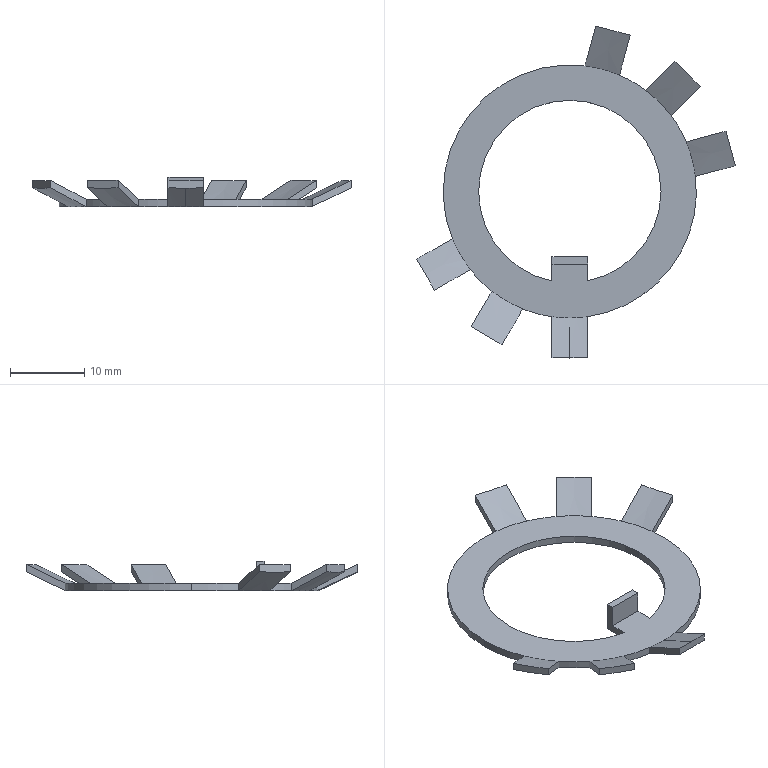Part | SolidWorks | features Boss 1, Cut 1, Revolution 1 | 1 solid | 49 faces | box 42.805 x 44.602 x 4 mm | volume 623.641 mm3 | plane 25 | cone 14 | cylinder 10 | commonest cylinder face diameters 34 x7 24.5 x3
STEP:
#1=CARTESIAN_POINT('',(0.,-17.,0.));
#2=VERTEX_POINT('',#1);
#3=CARTESIAN_POINT('',(-2.4,-16.83,0.));
#4=VERTEX_POINT('',#3);
#5=CARTESIAN_POINT('',(0.,0.,0.));
#6=DIRECTION('',(0.,0.,-1.));
#7=DIRECTION('',(0.,1.,0.));
#8=AXIS2_PLACEMENT_3D('',#5,#6,#7);
#9=CIRCLE('',#8,17.);
#10=EDGE_CURVE('',#2,#4,#9,.T.);
#11=ORIENTED_EDGE('',*,*,#10,.F.);
#12=CARTESIAN_POINT('',(0.,-22.372,2.505));
#13=VERTEX_POINT('',#12);
#14=CARTESIAN_POINT('',(0.,-17.,0.));
#15=DIRECTION('',(0.,-0.9063,0.4226));
#16=VECTOR('',#15,1000.);
#17=LINE('',#14,#16);
#18=EDGE_CURVE('',#2,#13,#17,.T.);
#19=ORIENTED_EDGE('',*,*,#18,.T.);
#20=CARTESIAN_POINT('',(-2.4,-22.372,2.565));
#21=VERTEX_POINT('',#20);
#22=CARTESIAN_POINT('',(0.,-22.372,2.505));
#23=CARTESIAN_POINT('',(-0.7988,-22.372,2.505));
#24=CARTESIAN_POINT('',(-1.6,-22.372,2.525));
#25=CARTESIAN_POINT('',(-2.4,-22.372,2.565));
#26=B_SPLINE_CURVE_WITH_KNOTS('',3,(#22,#23,#24,#25),.UNSPECIFIED.,.F.,.F.,(4,4),(0.00905,0.01144),.UNSPECIFIED.);
#27=EDGE_CURVE('',#13,#21,#26,.T.);
#28=ORIENTED_EDGE('',*,*,#27,.T.);
#29=CARTESIAN_POINT('',(-2.4,-22.372,2.565));
#30=CARTESIAN_POINT('',(-2.4,-20.525,1.708));
#31=CARTESIAN_POINT('',(-2.4,-18.678,0.8532));
#32=CARTESIAN_POINT('',(-2.4,-16.83,0.));
#33=B_SPLINE_CURVE_WITH_KNOTS('',3,(#29,#30,#31,#32),.UNSPECIFIED.,.F.,.F.,(4,4),(0.01129,0.01739),.UNSPECIFIED.);
#34=EDGE_CURVE('',#21,#4,#33,.T.);
#35=ORIENTED_EDGE('',*,*,#34,.T.);
#36=EDGE_LOOP('',(#11,#19,#28,#35));
#37=FACE_OUTER_BOUND('',#36,.T.);
#38=CARTESIAN_POINT('',(0.,0.,0.));
#39=DIRECTION('',(0.,0.,1.));
#40=DIRECTION('',(0.,-1.,0.));
#41=AXIS2_PLACEMENT_3D('',#38,#39,#40);
#42=CONICAL_SURFACE('',#41,17.,1.134);
#43=ADVANCED_FACE('',(#37),#42,.T.);
#44=CARTESIAN_POINT('',(-15.775,-6.336,1.));
#45=VERTEX_POINT('',#44);
#46=CARTESIAN_POINT('',(-17.,0.,1.));
#47=VERTEX_POINT('',#46);
#48=CARTESIAN_POINT('',(0.,0.,1.));
#49=DIRECTION('',(0.,0.,-1.));
#50=DIRECTION('',(0.,1.,0.));
#51=AXIS2_PLACEMENT_3D('',#48,#49,#50);
#52=CIRCLE('',#51,17.);
#53=EDGE_CURVE('',#45,#47,#52,.T.);
#54=ORIENTED_EDGE('',*,*,#53,.T.);
#55=CARTESIAN_POINT('',(-17.,0.,0.));
#56=VERTEX_POINT('',#55);
#57=CARTESIAN_POINT('',(-17.,0.,3.566));
#58=DIRECTION('',(0.,0.,-1.));
#59=VECTOR('',#58,1000.);
#60=LINE('',#57,#59);
#61=EDGE_CURVE('',#47,#56,#60,.T.);
#62=ORIENTED_EDGE('',*,*,#61,.T.);
#63=CARTESIAN_POINT('',(-15.775,-6.336,0.));
#64=VERTEX_POINT('',#63);
#65=CARTESIAN_POINT('',(0.,0.,0.));
#66=DIRECTION('',(0.,0.,1.));
#67=DIRECTION('',(1.,0.,0.));
#68=AXIS2_PLACEMENT_3D('',#65,#66,#67);
#69=CIRCLE('',#68,17.);
#70=EDGE_CURVE('',#56,#64,#69,.T.);
#71=ORIENTED_EDGE('',*,*,#70,.T.);
#72=CARTESIAN_POINT('',(-15.775,-6.336,3.566));
#73=DIRECTION('',(0.,0.,-1.));
#74=VECTOR('',#73,1000.);
#75=LINE('',#72,#74);
#76=EDGE_CURVE('',#45,#64,#75,.T.);
#77=ORIENTED_EDGE('',*,*,#76,.F.);
#78=EDGE_LOOP('',(#54,#62,#71,#77));
#79=FACE_OUTER_BOUND('',#78,.T.);
#80=CARTESIAN_POINT('',(0.,0.,3.566));
#81=DIRECTION('',(0.,0.,-1.));
#82=DIRECTION('',(-1.,0.,0.));
#83=AXIS2_PLACEMENT_3D('',#80,#81,#82);
#84=CYLINDRICAL_SURFACE('',#83,17.);
#85=ADVANCED_FACE('',(#79),#84,.T.);
#86=CARTESIAN_POINT('',(2.4,-12.013,1.));
#87=VERTEX_POINT('',#86);
#88=CARTESIAN_POINT('',(12.25,0.,1.));
#89=VERTEX_POINT('',#88);
#90=CARTESIAN_POINT('',(0.,0.,1.));
#91=DIRECTION('',(0.,0.,1.));
#92=DIRECTION('',(0.,-1.,0.));
#93=AXIS2_PLACEMENT_3D('',#90,#91,#92);
#94=CIRCLE('',#93,12.25);
#95=EDGE_CURVE('',#87,#89,#94,.T.);
#96=ORIENTED_EDGE('',*,*,#95,.T.);
#97=CARTESIAN_POINT('',(12.25,0.,0.));
#98=VERTEX_POINT('',#97);
#99=CARTESIAN_POINT('',(12.25,0.,3.566));
#100=DIRECTION('',(0.,0.,-1.));
#101=VECTOR('',#100,1000.);
#102=LINE('',#99,#101);
#103=EDGE_CURVE('',#89,#98,#102,.T.);
#104=ORIENTED_EDGE('',*,*,#103,.T.);
#105=CARTESIAN_POINT('',(2.4,-12.013,0.));
#106=VERTEX_POINT('',#105);
#107=CARTESIAN_POINT('',(0.,0.,0.));
#108=DIRECTION('',(0.,0.,1.));
#109=DIRECTION('',(1.,0.,0.));
#110=AXIS2_PLACEMENT_3D('',#107,#108,#109);
#111=CIRCLE('',#110,12.25);
#112=EDGE_CURVE('',#106,#98,#111,.T.);
#113=ORIENTED_EDGE('',*,*,#112,.F.);
#114=CARTESIAN_POINT('',(2.4,-12.013,3.566));
#115=DIRECTION('',(0.,0.,-1.));
#116=VECTOR('',#115,1000.);
#117=LINE('',#114,#116);
#118=EDGE_CURVE('',#87,#106,#117,.T.);
#119=ORIENTED_EDGE('',*,*,#118,.F.);
#120=EDGE_LOOP('',(#96,#104,#113,#119));
#121=FACE_OUTER_BOUND('',#120,.T.);
#122=CARTESIAN_POINT('',(0.,0.,3.566));
#123=DIRECTION('',(0.,0.,-1.));
#124=DIRECTION('',(-1.,0.,0.));
#125=AXIS2_PLACEMENT_3D('',#122,#123,#124);
#126=CYLINDRICAL_SURFACE('',#125,12.25);
#127=ADVANCED_FACE('',(#121),#126,.F.);
#128=ORIENTED_EDGE('',*,*,#103,.F.);
#129=CARTESIAN_POINT('',(-12.25,0.,1.));
#130=VERTEX_POINT('',#129);
#131=CARTESIAN_POINT('',(0.,0.,1.));
#132=DIRECTION('',(0.,0.,1.));
#133=DIRECTION('',(0.,-1.,0.));
#134=AXIS2_PLACEMENT_3D('',#131,#132,#133);
#135=CIRCLE('',#134,12.25);
#136=EDGE_CURVE('',#89,#130,#135,.T.);
#137=ORIENTED_EDGE('',*,*,#136,.T.);
#138=CARTESIAN_POINT('',(-12.25,0.,0.));
#139=VERTEX_POINT('',#138);
#140=CARTESIAN_POINT('',(-12.25,0.,3.566));
#141=DIRECTION('',(0.,0.,-1.));
#142=VECTOR('',#141,1000.);
#143=LINE('',#140,#142);
#144=EDGE_CURVE('',#130,#139,#143,.T.);
#145=ORIENTED_EDGE('',*,*,#144,.T.);
#146=CARTESIAN_POINT('',(0.,0.,0.));
#147=DIRECTION('',(0.,0.,1.));
#148=DIRECTION('',(1.,0.,0.));
#149=AXIS2_PLACEMENT_3D('',#146,#147,#148);
#150=CIRCLE('',#149,12.25);
#151=EDGE_CURVE('',#98,#139,#150,.T.);
#152=ORIENTED_EDGE('',*,*,#151,.F.);
#153=EDGE_LOOP('',(#128,#137,#145,#152));
#154=FACE_OUTER_BOUND('',#153,.T.);
#155=CARTESIAN_POINT('',(0.,0.,3.566));
#156=DIRECTION('',(0.,0.,-1.));
#157=DIRECTION('',(-1.,0.,0.));
#158=AXIS2_PLACEMENT_3D('',#155,#156,#157);
#159=CYLINDRICAL_SURFACE('',#158,12.25);
#160=ADVANCED_FACE('',(#154),#159,.F.);
#161=CARTESIAN_POINT('',(2.4,-16.83,1.));
#162=VERTEX_POINT('',#161);
#163=CARTESIAN_POINT('',(0.,-17.,1.));
#164=VERTEX_POINT('',#163);
#165=CARTESIAN_POINT('',(0.,0.,1.));
#166=DIRECTION('',(0.,0.,-1.));
#167=DIRECTION('',(0.,1.,0.));
#168=AXIS2_PLACEMENT_3D('',#165,#166,#167);
#169=CIRCLE('',#168,17.);
#170=EDGE_CURVE('',#162,#164,#169,.T.);
#171=ORIENTED_EDGE('',*,*,#170,.T.);
#172=CARTESIAN_POINT('',(0.,-22.372,3.505));
#173=VERTEX_POINT('',#172);
#174=CARTESIAN_POINT('',(0.,-22.5,3.565));
#175=DIRECTION('',(0.,-0.9063,0.4226));
#176=VECTOR('',#175,1000.);
#177=LINE('',#174,#176);
#178=EDGE_CURVE('',#164,#173,#177,.T.);
#179=ORIENTED_EDGE('',*,*,#178,.T.);
#180=CARTESIAN_POINT('',(2.4,-22.372,3.565));
#181=VERTEX_POINT('',#180);
#182=CARTESIAN_POINT('',(0.,-22.372,3.505));
#183=CARTESIAN_POINT('',(0.8014,-22.372,3.505));
#184=CARTESIAN_POINT('',(1.601,-22.372,3.525));
#185=CARTESIAN_POINT('',(2.4,-22.372,3.565));
#186=B_SPLINE_CURVE_WITH_KNOTS('',3,(#182,#183,#184,#185),.UNSPECIFIED.,.F.,.F.,(4,4),(0.01258,0.01498),.UNSPECIFIED.);
#187=EDGE_CURVE('',#173,#181,#186,.T.);
#188=ORIENTED_EDGE('',*,*,#187,.T.);
#189=CARTESIAN_POINT('',(2.4,-22.372,3.565));
#190=CARTESIAN_POINT('',(2.4,-20.525,2.708));
#191=CARTESIAN_POINT('',(2.4,-18.678,1.853));
#192=CARTESIAN_POINT('',(2.4,-16.83,1.));
#193=B_SPLINE_CURVE_WITH_KNOTS('',3,(#189,#190,#191,#192),.UNSPECIFIED.,.F.,.F.,(4,4),(0.01129,0.01739),.UNSPECIFIED.);
#194=EDGE_CURVE('',#181,#162,#193,.T.);
#195=ORIENTED_EDGE('',*,*,#194,.T.);
#196=EDGE_LOOP('',(#171,#179,#188,#195));
#197=FACE_OUTER_BOUND('',#196,.T.);
#198=CARTESIAN_POINT('',(0.,0.,3.565));
#199=DIRECTION('',(0.,0.,1.));
#200=DIRECTION('',(0.,-1.,0.));
#201=AXIS2_PLACEMENT_3D('',#198,#199,#200);
#202=CONICAL_SURFACE('',#201,22.5,1.134);
#203=ADVANCED_FACE('',(#197),#202,.F.);
#204=CARTESIAN_POINT('',(2.038,16.877,1.));
#205=VERTEX_POINT('',#204);
#206=CARTESIAN_POINT('',(6.674,15.635,1.));
#207=VERTEX_POINT('',#206);
#208=CARTESIAN_POINT('',(0.,0.,1.));
#209=DIRECTION('',(0.,0.,-1.));
#210=DIRECTION('',(0.,1.,0.));
#211=AXIS2_PLACEMENT_3D('',#208,#209,#210);
#212=CIRCLE('',#211,17.);
#213=EDGE_CURVE('',#205,#207,#212,.T.);
#214=ORIENTED_EDGE('',*,*,#213,.F.);
#215=CARTESIAN_POINT('',(0.,0.,1.));
#216=DIRECTION('',(0.,0.,-1.));
#217=DIRECTION('',(0.,1.,0.));
#218=AXIS2_PLACEMENT_3D('',#215,#216,#217);
#219=CIRCLE('',#218,17.);
#220=EDGE_CURVE('',#47,#205,#219,.T.);
#221=ORIENTED_EDGE('',*,*,#220,.F.);
#222=ORIENTED_EDGE('',*,*,#53,.F.);
#223=CARTESIAN_POINT('',(-13.375,-10.493,1.));
#224=VERTEX_POINT('',#223);
#225=CARTESIAN_POINT('',(0.,0.,1.));
#226=DIRECTION('',(0.,0.,-1.));
#227=DIRECTION('',(0.,1.,0.));
#228=AXIS2_PLACEMENT_3D('',#225,#226,#227);
#229=CIRCLE('',#228,17.);
#230=EDGE_CURVE('',#224,#45,#229,.T.);
#231=ORIENTED_EDGE('',*,*,#230,.F.);
#232=CARTESIAN_POINT('',(-10.493,-13.375,1.));
#233=VERTEX_POINT('',#232);
#234=CARTESIAN_POINT('',(0.,0.,1.));
#235=DIRECTION('',(0.,0.,-1.));
#236=DIRECTION('',(0.,1.,0.));
#237=AXIS2_PLACEMENT_3D('',#234,#235,#236);
#238=CIRCLE('',#237,17.);
#239=EDGE_CURVE('',#233,#224,#238,.T.);
#240=ORIENTED_EDGE('',*,*,#239,.F.);
#241=CARTESIAN_POINT('',(-6.336,-15.775,1.));
#242=VERTEX_POINT('',#241);
#243=CARTESIAN_POINT('',(0.,0.,1.));
#244=DIRECTION('',(0.,0.,-1.));
#245=DIRECTION('',(0.,1.,0.));
#246=AXIS2_PLACEMENT_3D('',#243,#244,#245);
#247=CIRCLE('',#246,17.);
#248=EDGE_CURVE('',#242,#233,#247,.T.);
#249=ORIENTED_EDGE('',*,*,#248,.F.);
#250=CARTESIAN_POINT('',(-2.4,-16.83,1.));
#251=VERTEX_POINT('',#250);
#252=CARTESIAN_POINT('',(0.,0.,1.));
#253=DIRECTION('',(0.,0.,-1.));
#254=DIRECTION('',(0.,1.,0.));
#255=AXIS2_PLACEMENT_3D('',#252,#253,#254);
#256=CIRCLE('',#255,17.);
#257=EDGE_CURVE('',#251,#242,#256,.T.);
#258=ORIENTED_EDGE('',*,*,#257,.F.);
#259=CARTESIAN_POINT('',(0.,0.,1.));
#260=DIRECTION('',(0.,0.,-1.));
#261=DIRECTION('',(0.,1.,0.));
#262=AXIS2_PLACEMENT_3D('',#259,#260,#261);
#263=CIRCLE('',#262,17.);
#264=EDGE_CURVE('',#164,#251,#263,.T.);
#265=ORIENTED_EDGE('',*,*,#264,.F.);
#266=ORIENTED_EDGE('',*,*,#170,.F.);
#267=CARTESIAN_POINT('',(16.877,2.038,1.));
#268=VERTEX_POINT('',#267);
#269=CARTESIAN_POINT('',(0.,0.,1.));
#270=DIRECTION('',(0.,0.,-1.));
#271=DIRECTION('',(0.,1.,0.));
#272=AXIS2_PLACEMENT_3D('',#269,#270,#271);
#273=CIRCLE('',#272,17.);
#274=EDGE_CURVE('',#268,#162,#273,.T.);
#275=ORIENTED_EDGE('',*,*,#274,.F.);
#276=CARTESIAN_POINT('',(15.635,6.674,1.));
#277=VERTEX_POINT('',#276);
#278=CARTESIAN_POINT('',(0.,0.,1.));
#279=DIRECTION('',(0.,0.,-1.));
#280=DIRECTION('',(0.,1.,0.));
#281=AXIS2_PLACEMENT_3D('',#278,#279,#280);
#282=CIRCLE('',#281,17.);
#283=EDGE_CURVE('',#277,#268,#282,.T.);
#284=ORIENTED_EDGE('',*,*,#283,.F.);
#285=CARTESIAN_POINT('',(13.597,10.203,1.));
#286=VERTEX_POINT('',#285);
#287=CARTESIAN_POINT('',(0.,0.,1.));
#288=DIRECTION('',(0.,0.,-1.));
#289=DIRECTION('',(0.,1.,0.));
#290=AXIS2_PLACEMENT_3D('',#287,#288,#289);
#291=CIRCLE('',#290,17.);
#292=EDGE_CURVE('',#286,#277,#291,.T.);
#293=ORIENTED_EDGE('',*,*,#292,.F.);
#294=CARTESIAN_POINT('',(10.203,13.597,1.));
#295=VERTEX_POINT('',#294);
#296=CARTESIAN_POINT('',(0.,0.,1.));
#297=DIRECTION('',(0.,0.,-1.));
#298=DIRECTION('',(0.,1.,0.));
#299=AXIS2_PLACEMENT_3D('',#296,#297,#298);
#300=CIRCLE('',#299,17.);
#301=EDGE_CURVE('',#295,#286,#300,.T.);
#302=ORIENTED_EDGE('',*,*,#301,.F.);
#303=CARTESIAN_POINT('',(0.,0.,1.));
#304=DIRECTION('',(0.,0.,-1.));
#305=DIRECTION('',(0.,1.,0.));
#306=AXIS2_PLACEMENT_3D('',#303,#304,#305);
#307=CIRCLE('',#306,17.);
#308=EDGE_CURVE('',#207,#295,#307,.T.);
#309=ORIENTED_EDGE('',*,*,#308,.F.);
#310=EDGE_LOOP('',(#214,#221,#222,#231,#240,#249,#258,#265,#266,#275,#284,#293,#302,#309));
#311=FACE_OUTER_BOUND('',#310,.T.);
#312=CARTESIAN_POINT('',(2.4,-9.75,1.));
#313=VERTEX_POINT('',#312);
#314=CARTESIAN_POINT('',(2.4,-12.013,1.));
#315=DIRECTION('',(0.,-1.,0.));
#316=VECTOR('',#315,1000.);
#317=LINE('',#314,#316);
#318=EDGE_CURVE('',#313,#87,#317,.T.);
#319=ORIENTED_EDGE('',*,*,#318,.F.);
#320=CARTESIAN_POINT('',(-2.4,-9.75,1.));
#321=VERTEX_POINT('',#320);
#322=CARTESIAN_POINT('',(0.,-9.75,1.));
#323=DIRECTION('',(-1.,0.,0.));
#324=VECTOR('',#323,1000.);
#325=LINE('',#322,#324);
#326=EDGE_CURVE('',#313,#321,#325,.T.);
#327=ORIENTED_EDGE('',*,*,#326,.T.);
#328=CARTESIAN_POINT('',(-2.4,-12.013,1.));
#329=VERTEX_POINT('',#328);
#330=CARTESIAN_POINT('',(-2.4,-12.013,1.));
#331=DIRECTION('',(0.,1.,0.));
#332=VECTOR('',#331,1000.);
#333=LINE('',#330,#332);
#334=EDGE_CURVE('',#329,#321,#333,.T.);
#335=ORIENTED_EDGE('',*,*,#334,.F.);
#336=CARTESIAN_POINT('',(0.,0.,1.));
#337=DIRECTION('',(0.,0.,1.));
#338=DIRECTION('',(0.,-1.,0.));
#339=AXIS2_PLACEMENT_3D('',#336,#337,#338);
#340=CIRCLE('',#339,12.25);
#341=EDGE_CURVE('',#130,#329,#340,.T.);
#342=ORIENTED_EDGE('',*,*,#341,.F.);
#343=ORIENTED_EDGE('',*,*,#136,.F.);
#344=ORIENTED_EDGE('',*,*,#95,.F.);
#345=EDGE_LOOP('',(#319,#327,#335,#342,#343,#344));
#346=FACE_BOUND('',#345,.T.);
#347=CARTESIAN_POINT('',(0.,17.,1.));
#348=DIRECTION('',(0.,0.,1.));
#349=DIRECTION('',(0.,-1.,0.));
#350=AXIS2_PLACEMENT_3D('',#347,#348,#349);
#351=PLANE('',#350);
#352=ADVANCED_FACE('',(#311,#346),#351,.T.);
#353=ORIENTED_EDGE('',*,*,#178,.F.);
#354=ORIENTED_EDGE('',*,*,#264,.T.);
#355=CARTESIAN_POINT('',(-2.4,-22.372,3.565));
#356=VERTEX_POINT('',#355);
#357=CARTESIAN_POINT('',(-2.4,-16.83,1.));
#358=CARTESIAN_POINT('',(-2.4,-18.678,1.853));
#359=CARTESIAN_POINT('',(-2.4,-20.525,2.708));
#360=CARTESIAN_POINT('',(-2.4,-22.372,3.565));
#361=B_SPLINE_CURVE_WITH_KNOTS('',3,(#357,#358,#359,#360),.UNSPECIFIED.,.F.,.F.,(4,4),(0.006977,0.01308),.UNSPECIFIED.);
#362=EDGE_CURVE('',#251,#356,#361,.T.);
#363=ORIENTED_EDGE('',*,*,#362,.T.);
#364=CARTESIAN_POINT('',(-2.4,-22.372,3.565));
#365=CARTESIAN_POINT('',(-1.6,-22.372,3.525));
#366=CARTESIAN_POINT('',(-0.7988,-22.372,3.505));
#367=CARTESIAN_POINT('',(0.,-22.372,3.505));
#368=B_SPLINE_CURVE_WITH_KNOTS('',3,(#364,#365,#366,#367),.UNSPECIFIED.,.F.,.F.,(4,4),(0.01019,0.01258),.UNSPECIFIED.);
#369=EDGE_CURVE('',#356,#173,#368,.T.);
#370=ORIENTED_EDGE('',*,*,#369,.T.);
#371=EDGE_LOOP('',(#353,#354,#363,#370));
#372=FACE_OUTER_BOUND('',#371,.T.);
#373=CARTESIAN_POINT('',(0.,0.,3.565));
#374=DIRECTION('',(0.,0.,1.));
#375=DIRECTION('',(0.,-1.,0.));
#376=AXIS2_PLACEMENT_3D('',#373,#374,#375);
#377=CONICAL_SURFACE('',#376,22.5,1.134);
#378=ADVANCED_FACE('',(#372),#377,.F.);
#379=CARTESIAN_POINT('',(-13.264,-18.174,3.565));
#380=VERTEX_POINT('',#379);
#381=CARTESIAN_POINT('',(-10.493,-13.375,1.));
#382=CARTESIAN_POINT('',(-11.417,-14.975,1.853));
#383=CARTESIAN_POINT('',(-12.341,-16.575,2.708));
#384=CARTESIAN_POINT('',(-13.264,-18.174,3.565));
#385=B_SPLINE_CURVE_WITH_KNOTS('',3,(#381,#382,#383,#384),.UNSPECIFIED.,.F.,.F.,(4,4),(0.000000254,0.006107),.UNSPECIFIED.);
#386=EDGE_CURVE('',#233,#380,#385,.T.);
#387=ORIENTED_EDGE('',*,*,#386,.T.);
#388=CARTESIAN_POINT('',(-9.107,-20.574,3.565));
#389=VERTEX_POINT('',#388);
#390=CARTESIAN_POINT('',(-13.264,-18.174,3.565));
#391=CARTESIAN_POINT('',(-11.879,-18.974,3.485));
#392=CARTESIAN_POINT('',(-10.493,-19.774,3.485));
#393=CARTESIAN_POINT('',(-9.107,-20.574,3.565));
#394=B_SPLINE_CURVE_WITH_KNOTS('',3,(#390,#391,#392,#393),.UNSPECIFIED.,.F.,.F.,(4,4),(0.000000231,0.0048),.UNSPECIFIED.);
#395=EDGE_CURVE('',#380,#389,#394,.T.);
#396=ORIENTED_EDGE('',*,*,#395,.T.);
#397=CARTESIAN_POINT('',(-9.107,-20.574,3.565));
#398=CARTESIAN_POINT('',(-8.184,-18.975,2.708));
#399=CARTESIAN_POINT('',(-7.26,-17.375,1.853));
#400=CARTESIAN_POINT('',(-6.336,-15.775,1.));
#401=B_SPLINE_CURVE_WITH_KNOTS('',3,(#397,#398,#399,#400),.UNSPECIFIED.,.F.,.F.,(4,4),(0.000000255,0.006107),.UNSPECIFIED.);
#402=EDGE_CURVE('',#389,#242,#401,.T.);
#403=ORIENTED_EDGE('',*,*,#402,.T.);
#404=ORIENTED_EDGE('',*,*,#248,.T.);
#405=EDGE_LOOP('',(#387,#396,#403,#404));
#406=FACE_OUTER_BOUND('',#405,.T.);
#407=CARTESIAN_POINT('',(0.,0.,3.565));
#408=DIRECTION('',(0.,0.,1.));
#409=DIRECTION('',(0.,-1.,0.));
#410=AXIS2_PLACEMENT_3D('',#407,#408,#409);
#411=CONICAL_SURFACE('',#410,22.5,1.134);
#412=ADVANCED_FACE('',(#406),#411,.F.);
#413=CARTESIAN_POINT('',(-20.574,-9.107,3.565));
#414=VERTEX_POINT('',#413);
#415=CARTESIAN_POINT('',(-15.775,-6.336,1.));
#416=CARTESIAN_POINT('',(-17.375,-7.26,1.853));
#417=CARTESIAN_POINT('',(-18.975,-8.184,2.708));
#418=CARTESIAN_POINT('',(-20.574,-9.107,3.565));
#419=B_SPLINE_CURVE_WITH_KNOTS('',3,(#415,#416,#417,#418),.UNSPECIFIED.,.F.,.F.,(4,4),(0.000000254,0.006107),.UNSPECIFIED.);
#420=EDGE_CURVE('',#45,#414,#419,.T.);
#421=ORIENTED_EDGE('',*,*,#420,.T.);
#422=CARTESIAN_POINT('',(-18.174,-13.264,3.565));
#423=VERTEX_POINT('',#422);
#424=CARTESIAN_POINT('',(-20.574,-9.107,3.565));
#425=CARTESIAN_POINT('',(-19.774,-10.493,3.485));
#426=CARTESIAN_POINT('',(-18.974,-11.879,3.485));
#427=CARTESIAN_POINT('',(-18.174,-13.264,3.565));
#428=B_SPLINE_CURVE_WITH_KNOTS('',3,(#424,#425,#426,#427),.UNSPECIFIED.,.F.,.F.,(4,4),(0.000000231,0.0048),.UNSPECIFIED.);
#429=EDGE_CURVE('',#414,#423,#428,.T.);
#430=ORIENTED_EDGE('',*,*,#429,.T.);
#431=CARTESIAN_POINT('',(-18.174,-13.264,3.565));
#432=CARTESIAN_POINT('',(-16.575,-12.341,2.708));
#433=CARTESIAN_POINT('',(-14.975,-11.417,1.853));
#434=CARTESIAN_POINT('',(-13.375,-10.493,1.));
#435=B_SPLINE_CURVE_WITH_KNOTS('',3,(#431,#432,#433,#434),.UNSPECIFIED.,.F.,.F.,(4,4),(0.000000255,0.006107),.UNSPECIFIED.);
#436=EDGE_CURVE('',#423,#224,#435,.T.);
#437=ORIENTED_EDGE('',*,*,#436,.T.);
#438=ORIENTED_EDGE('',*,*,#230,.T.);
#439=EDGE_LOOP('',(#421,#430,#437,#438));
#440=FACE_OUTER_BOUND('',#439,.T.);
#441=CARTESIAN_POINT('',(0.,0.,3.565));
#442=DIRECTION('',(0.,0.,1.));
#443=DIRECTION('',(0.,-1.,0.));
#444=AXIS2_PLACEMENT_3D('',#441,#442,#443);
#445=CONICAL_SURFACE('',#444,22.5,1.134);
#446=ADVANCED_FACE('',(#440),#445,.F.);
#447=CARTESIAN_POINT('',(8.108,20.988,3.565));
#448=VERTEX_POINT('',#447);
#449=CARTESIAN_POINT('',(6.674,15.635,1.));
#450=CARTESIAN_POINT('',(7.152,17.42,1.853));
#451=CARTESIAN_POINT('',(7.63,19.204,2.708));
#452=CARTESIAN_POINT('',(8.108,20.988,3.565));
#453=B_SPLINE_CURVE_WITH_KNOTS('',3,(#449,#450,#451,#452),.UNSPECIFIED.,.F.,.F.,(4,4),(0.000000228,0.006107),.UNSPECIFIED.);
#454=EDGE_CURVE('',#207,#448,#453,.T.);
#455=ORIENTED_EDGE('',*,*,#454,.T.);
#456=CARTESIAN_POINT('',(3.472,22.231,3.565));
#457=VERTEX_POINT('',#456);
#458=CARTESIAN_POINT('',(8.108,20.988,3.565));
#459=CARTESIAN_POINT('',(6.563,21.402,3.485));
#460=CARTESIAN_POINT('',(5.017,21.816,3.485));
#461=CARTESIAN_POINT('',(3.472,22.231,3.565));
#462=B_SPLINE_CURVE_WITH_KNOTS('',3,(#458,#459,#460,#461),.UNSPECIFIED.,.F.,.F.,(4,4),(0.000000207,0.0048),.UNSPECIFIED.);
#463=EDGE_CURVE('',#448,#457,#462,.T.);
#464=ORIENTED_EDGE('',*,*,#463,.T.);
#465=CARTESIAN_POINT('',(3.472,22.231,3.565));
#466=CARTESIAN_POINT('',(2.994,20.447,2.708));
#467=CARTESIAN_POINT('',(2.516,18.663,1.853));
#468=CARTESIAN_POINT('',(2.038,16.877,1.));
#469=B_SPLINE_CURVE_WITH_KNOTS('',3,(#465,#466,#467,#468),.UNSPECIFIED.,.F.,.F.,(4,4),(0.000000228,0.006107),.UNSPECIFIED.);
#470=EDGE_CURVE('',#457,#205,#469,.T.);
#471=ORIENTED_EDGE('',*,*,#470,.T.);
#472=ORIENTED_EDGE('',*,*,#213,.T.);
#473=EDGE_LOOP('',(#455,#464,#471,#472));
#474=FACE_OUTER_BOUND('',#473,.T.);
#475=CARTESIAN_POINT('',(0.,0.,3.565));
#476=DIRECTION('',(0.,0.,1.));
#477=DIRECTION('',(0.,-1.,0.));
#478=AXIS2_PLACEMENT_3D('',#475,#476,#477);
#479=CONICAL_SURFACE('',#478,22.5,1.134);
#480=ADVANCED_FACE('',(#474),#479,.F.);
#481=CARTESIAN_POINT('',(17.516,14.122,3.565));
#482=VERTEX_POINT('',#481);
#483=CARTESIAN_POINT('',(13.597,10.203,1.));
#484=CARTESIAN_POINT('',(14.904,11.51,1.853));
#485=CARTESIAN_POINT('',(16.21,12.816,2.708));
#486=CARTESIAN_POINT('',(17.516,14.122,3.565));
#487=B_SPLINE_CURVE_WITH_KNOTS('',3,(#483,#484,#485,#486),.UNSPECIFIED.,.F.,.F.,(4,4),(0.000000312,0.006107),.UNSPECIFIED.);
#488=EDGE_CURVE('',#286,#482,#487,.T.);
#489=ORIENTED_EDGE('',*,*,#488,.T.);
#490=CARTESIAN_POINT('',(14.122,17.516,3.565));
#491=VERTEX_POINT('',#490);
#492=CARTESIAN_POINT('',(17.516,14.122,3.565));
#493=CARTESIAN_POINT('',(16.385,15.253,3.485));
#494=CARTESIAN_POINT('',(15.253,16.385,3.485));
#495=CARTESIAN_POINT('',(14.122,17.516,3.565));
#496=B_SPLINE_CURVE_WITH_KNOTS('',3,(#492,#493,#494,#495),.UNSPECIFIED.,.F.,.F.,(4,4),(0.000000283,0.0048),.UNSPECIFIED.);
#497=EDGE_CURVE('',#482,#491,#496,.T.);
#498=ORIENTED_EDGE('',*,*,#497,.T.);
#499=CARTESIAN_POINT('',(14.122,17.516,3.565));
#500=CARTESIAN_POINT('',(12.816,16.21,2.708));
#501=CARTESIAN_POINT('',(11.51,14.904,1.853));
#502=CARTESIAN_POINT('',(10.203,13.597,1.));
#503=B_SPLINE_CURVE_WITH_KNOTS('',3,(#499,#500,#501,#502),.UNSPECIFIED.,.F.,.F.,(4,4),(0.000000312,0.006107),.UNSPECIFIED.);
#504=EDGE_CURVE('',#491,#295,#503,.T.);
#505=ORIENTED_EDGE('',*,*,#504,.T.);
#506=ORIENTED_EDGE('',*,*,#301,.T.);
#507=EDGE_LOOP('',(#489,#498,#505,#506));
#508=FACE_OUTER_BOUND('',#507,.T.);
#509=CARTESIAN_POINT('',(0.,0.,3.565));
#510=DIRECTION('',(0.,0.,1.));
#511=DIRECTION('',(0.,-1.,0.));
#512=AXIS2_PLACEMENT_3D('',#509,#510,#511);
#513=CONICAL_SURFACE('',#512,22.5,1.134);
#514=ADVANCED_FACE('',(#508),#513,.F.);
#515=CARTESIAN_POINT('',(22.231,3.472,3.565));
#516=VERTEX_POINT('',#515);
#517=CARTESIAN_POINT('',(16.877,2.038,1.));
#518=CARTESIAN_POINT('',(18.663,2.516,1.853));
#519=CARTESIAN_POINT('',(20.447,2.994,2.708));
#520=CARTESIAN_POINT('',(22.231,3.472,3.565));
#521=B_SPLINE_CURVE_WITH_KNOTS('',3,(#517,#518,#519,#520),.UNSPECIFIED.,.F.,.F.,(4,4),(0.000000228,0.006107),.UNSPECIFIED.);
#522=EDGE_CURVE('',#268,#516,#521,.T.);
#523=ORIENTED_EDGE('',*,*,#522,.T.);
#524=CARTESIAN_POINT('',(20.988,8.108,3.565));
#525=VERTEX_POINT('',#524);
#526=CARTESIAN_POINT('',(22.231,3.472,3.565));
#527=CARTESIAN_POINT('',(21.816,5.017,3.485));
#528=CARTESIAN_POINT('',(21.402,6.563,3.485));
#529=CARTESIAN_POINT('',(20.988,8.108,3.565));
#530=B_SPLINE_CURVE_WITH_KNOTS('',3,(#526,#527,#528,#529),.UNSPECIFIED.,.F.,.F.,(4,4),(0.000000207,0.0048),.UNSPECIFIED.);
#531=EDGE_CURVE('',#516,#525,#530,.T.);
#532=ORIENTED_EDGE('',*,*,#531,.T.);
#533=CARTESIAN_POINT('',(20.988,8.108,3.565));
#534=CARTESIAN_POINT('',(19.204,7.63,2.708));
#535=CARTESIAN_POINT('',(17.42,7.152,1.853));
#536=CARTESIAN_POINT('',(15.635,6.674,1.));
#537=B_SPLINE_CURVE_WITH_KNOTS('',3,(#533,#534,#535,#536),.UNSPECIFIED.,.F.,.F.,(4,4),(0.000000228,0.006107),.UNSPECIFIED.);
#538=EDGE_CURVE('',#525,#277,#537,.T.);
#539=ORIENTED_EDGE('',*,*,#538,.T.);
#540=ORIENTED_EDGE('',*,*,#283,.T.);
#541=EDGE_LOOP('',(#523,#532,#539,#540));
#542=FACE_OUTER_BOUND('',#541,.T.);
#543=CARTESIAN_POINT('',(0.,0.,3.565));
#544=DIRECTION('',(0.,0.,1.));
#545=DIRECTION('',(0.,-1.,0.));
#546=AXIS2_PLACEMENT_3D('',#543,#544,#545);
#547=CONICAL_SURFACE('',#546,22.5,1.134);
#548=ADVANCED_FACE('',(#542),#547,.F.);
#549=CARTESIAN_POINT('',(2.4,-8.75,4.));
#550=VERTEX_POINT('',#549);
#551=CARTESIAN_POINT('',(2.4,-8.75,0.));
#552=VERTEX_POINT('',#551);
#553=CARTESIAN_POINT('',(2.4,-8.75,3.566));
#554=DIRECTION('',(0.,0.,-1.));
#555=VECTOR('',#554,1000.);
#556=LINE('',#553,#555);
#557=EDGE_CURVE('',#550,#552,#556,.T.);
#558=ORIENTED_EDGE('',*,*,#557,.F.);
#559=CARTESIAN_POINT('',(2.4,-9.75,4.));
#560=VERTEX_POINT('',#559);
#561=CARTESIAN_POINT('',(2.4,-8.75,4.));
#562=DIRECTION('',(0.,1.,0.));
#563=VECTOR('',#562,1000.);
#564=LINE('',#561,#563);
#565=EDGE_CURVE('',#560,#550,#564,.T.);
#566=ORIENTED_EDGE('',*,*,#565,.F.);
#567=CARTESIAN_POINT('',(2.4,-9.75,4.));
#568=DIRECTION('',(0.,0.,-1.));
#569=VECTOR('',#568,1000.);
#570=LINE('',#567,#569);
#571=EDGE_CURVE('',#560,#313,#570,.T.);
#572=ORIENTED_EDGE('',*,*,#571,.T.);
#573=ORIENTED_EDGE('',*,*,#318,.T.);
#574=ORIENTED_EDGE('',*,*,#118,.T.);
#575=CARTESIAN_POINT('',(2.4,-12.013,0.));
#576=DIRECTION('',(0.,-1.,0.));
#577=VECTOR('',#576,1000.);
#578=LINE('',#575,#577);
#579=EDGE_CURVE('',#552,#106,#578,.T.);
#580=ORIENTED_EDGE('',*,*,#579,.F.);
#581=EDGE_LOOP('',(#558,#566,#572,#573,#574,#580));
#582=FACE_OUTER_BOUND('',#581,.T.);
#583=CARTESIAN_POINT('',(2.4,-12.013,3.566));
#584=DIRECTION('',(1.,0.,0.));
#585=DIRECTION('',(0.,0.,-1.));
#586=AXIS2_PLACEMENT_3D('',#583,#584,#585);
#587=PLANE('',#586);
#588=ADVANCED_FACE('',(#582),#587,.T.);
#589=CARTESIAN_POINT('',(-2.4,-8.75,4.));
#590=VERTEX_POINT('',#589);
#591=CARTESIAN_POINT('',(-2.4,-8.75,0.));
#592=VERTEX_POINT('',#591);
#593=CARTESIAN_POINT('',(-2.4,-8.75,3.566));
#594=DIRECTION('',(0.,0.,-1.));
#595=VECTOR('',#594,1000.);
#596=LINE('',#593,#595);
#597=EDGE_CURVE('',#590,#592,#596,.T.);
#598=ORIENTED_EDGE('',*,*,#597,.F.);
#599=CARTESIAN_POINT('',(-2.4,-8.75,4.));
#600=DIRECTION('',(-1.,0.,0.));
#601=VECTOR('',#600,1000.);
#602=LINE('',#599,#601);
#603=EDGE_CURVE('',#550,#590,#602,.T.);
#604=ORIENTED_EDGE('',*,*,#603,.F.);
#605=ORIENTED_EDGE('',*,*,#557,.T.);
#606=CARTESIAN_POINT('',(2.4,-8.75,0.));
#607=DIRECTION('',(1.,0.,0.));
#608=VECTOR('',#607,1000.);
#609=LINE('',#606,#608);
#610=EDGE_CURVE('',#592,#552,#609,.T.);
#611=ORIENTED_EDGE('',*,*,#610,.F.);
#612=EDGE_LOOP('',(#598,#604,#605,#611));
#613=FACE_OUTER_BOUND('',#612,.T.);
#614=CARTESIAN_POINT('',(2.4,-8.75,3.566));
#615=DIRECTION('',(0.,1.,0.));
#616=DIRECTION('',(0.,0.,1.));
#617=AXIS2_PLACEMENT_3D('',#614,#615,#616);
#618=PLANE('',#617);
#619=ADVANCED_FACE('',(#613),#618,.T.);
#620=ORIENTED_EDGE('',*,*,#597,.T.);
#621=CARTESIAN_POINT('',(-2.4,-12.013,0.));
#622=VERTEX_POINT('',#621);
#623=CARTESIAN_POINT('',(-2.4,-12.013,0.));
#624=DIRECTION('',(0.,1.,0.));
#625=VECTOR('',#624,1000.);
#626=LINE('',#623,#625);
#627=EDGE_CURVE('',#622,#592,#626,.T.);
#628=ORIENTED_EDGE('',*,*,#627,.F.);
#629=CARTESIAN_POINT('',(-2.4,-12.013,3.566));
#630=DIRECTION('',(0.,0.,-1.));
#631=VECTOR('',#630,1000.);
#632=LINE('',#629,#631);
#633=EDGE_CURVE('',#329,#622,#632,.T.);
#634=ORIENTED_EDGE('',*,*,#633,.F.);
#635=ORIENTED_EDGE('',*,*,#334,.T.);
#636=CARTESIAN_POINT('',(-2.4,-9.75,4.));
#637=VERTEX_POINT('',#636);
#638=CARTESIAN_POINT('',(-2.4,-9.75,4.));
#639=DIRECTION('',(0.,0.,-1.));
#640=VECTOR('',#639,1000.);
#641=LINE('',#638,#640);
#642=EDGE_CURVE('',#637,#321,#641,.T.);
#643=ORIENTED_EDGE('',*,*,#642,.F.);
#644=CARTESIAN_POINT('',(-2.4,-8.75,4.));
#645=DIRECTION('',(0.,-1.,0.));
#646=VECTOR('',#645,1000.);
#647=LINE('',#644,#646);
#648=EDGE_CURVE('',#590,#637,#647,.T.);
#649=ORIENTED_EDGE('',*,*,#648,.F.);
#650=EDGE_LOOP('',(#620,#628,#634,#635,#643,#649));
#651=FACE_OUTER_BOUND('',#650,.T.);
#652=CARTESIAN_POINT('',(-2.4,-12.013,3.566));
#653=DIRECTION('',(-1.,0.,0.));
#654=DIRECTION('',(0.,-1.,0.));
#655=AXIS2_PLACEMENT_3D('',#652,#653,#654);
#656=PLANE('',#655);
#657=ADVANCED_FACE('',(#651),#656,.T.);
#658=ORIENTED_EDGE('',*,*,#144,.F.);
#659=ORIENTED_EDGE('',*,*,#341,.T.);
#660=ORIENTED_EDGE('',*,*,#633,.T.);
#661=CARTESIAN_POINT('',(0.,0.,0.));
#662=DIRECTION('',(0.,0.,1.));
#663=DIRECTION('',(1.,0.,0.));
#664=AXIS2_PLACEMENT_3D('',#661,#662,#663);
#665=CIRCLE('',#664,12.25);
#666=EDGE_CURVE('',#139,#622,#665,.T.);
#667=ORIENTED_EDGE('',*,*,#666,.F.);
#668=EDGE_LOOP('',(#658,#659,#660,#667));
#669=FACE_OUTER_BOUND('',#668,.T.);
#670=CARTESIAN_POINT('',(0.,0.,3.566));
#671=DIRECTION('',(0.,0.,-1.));
#672=DIRECTION('',(-1.,0.,0.));
#673=AXIS2_PLACEMENT_3D('',#670,#671,#672);
#674=CYLINDRICAL_SURFACE('',#673,12.25);
#675=ADVANCED_FACE('',(#669),#674,.F.);
#676=CARTESIAN_POINT('',(2.4,-16.83,0.));
#677=VERTEX_POINT('',#676);
#678=CARTESIAN_POINT('',(2.4,-22.372,2.565));
#679=VERTEX_POINT('',#678);
#680=CARTESIAN_POINT('',(2.4,-16.83,0.));
#681=CARTESIAN_POINT('',(2.4,-18.678,0.8532));
#682=CARTESIAN_POINT('',(2.4,-20.525,1.708));
#683=CARTESIAN_POINT('',(2.4,-22.372,2.565));
#684=B_SPLINE_CURVE_WITH_KNOTS('',3,(#680,#681,#682,#683),.UNSPECIFIED.,.F.,.F.,(4,4),(0.006977,0.01308),.UNSPECIFIED.);
#685=EDGE_CURVE('',#677,#679,#684,.T.);
#686=ORIENTED_EDGE('',*,*,#685,.F.);
#687=CARTESIAN_POINT('',(2.4,-16.83,3.566));
#688=DIRECTION('',(0.,0.,-1.));
#689=VECTOR('',#688,1000.);
#690=LINE('',#687,#689);
#691=EDGE_CURVE('',#162,#677,#690,.T.);
#692=ORIENTED_EDGE('',*,*,#691,.F.);
#693=ORIENTED_EDGE('',*,*,#194,.F.);
#694=CARTESIAN_POINT('',(2.4,-22.372,3.566));
#695=DIRECTION('',(0.,0.,-1.));
#696=VECTOR('',#695,1000.);
#697=LINE('',#694,#696);
#698=EDGE_CURVE('',#181,#679,#697,.T.);
#699=ORIENTED_EDGE('',*,*,#698,.T.);
#700=EDGE_LOOP('',(#686,#692,#693,#699));
#701=FACE_OUTER_BOUND('',#700,.T.);
#702=CARTESIAN_POINT('',(2.4,-16.83,3.566));
#703=DIRECTION('',(-1.,0.,0.));
#704=DIRECTION('',(0.,-1.,0.));
#705=AXIS2_PLACEMENT_3D('',#702,#703,#704);
#706=PLANE('',#705);
#707=ADVANCED_FACE('',(#701),#706,.F.);
#708=ORIENTED_EDGE('',*,*,#274,.T.);
#709=ORIENTED_EDGE('',*,*,#691,.T.);
#710=CARTESIAN_POINT('',(16.877,2.038,0.));
#711=VERTEX_POINT('',#710);
#712=CARTESIAN_POINT('',(0.,0.,0.));
#713=DIRECTION('',(0.,0.,1.));
#714=DIRECTION('',(1.,0.,0.));
#715=AXIS2_PLACEMENT_3D('',#712,#713,#714);
#716=CIRCLE('',#715,17.);
#717=EDGE_CURVE('',#677,#711,#716,.T.);
#718=ORIENTED_EDGE('',*,*,#717,.T.);
#719=CARTESIAN_POINT('',(16.877,2.038,3.566));
#720=DIRECTION('',(0.,0.,-1.));
#721=VECTOR('',#720,1000.);
#722=LINE('',#719,#721);
#723=EDGE_CURVE('',#268,#711,#722,.T.);
#724=ORIENTED_EDGE('',*,*,#723,.F.);
#725=EDGE_LOOP('',(#708,#709,#718,#724));
#726=FACE_OUTER_BOUND('',#725,.T.);
#727=CARTESIAN_POINT('',(0.,0.,3.566));
#728=DIRECTION('',(0.,0.,-1.));
#729=DIRECTION('',(-1.,0.,0.));
#730=AXIS2_PLACEMENT_3D('',#727,#728,#729);
#731=CYLINDRICAL_SURFACE('',#730,17.);
#732=ADVANCED_FACE('',(#726),#731,.T.);
#733=CARTESIAN_POINT('',(22.231,3.472,2.565));
#734=VERTEX_POINT('',#733);
#735=CARTESIAN_POINT('',(22.231,3.472,2.565));
#736=CARTESIAN_POINT('',(20.447,2.994,1.708));
#737=CARTESIAN_POINT('',(18.663,2.516,0.8532));
#738=CARTESIAN_POINT('',(16.877,2.038,0.));
#739=B_SPLINE_CURVE_WITH_KNOTS('',3,(#735,#736,#737,#738),.UNSPECIFIED.,.F.,.F.,(4,4),(0.000000228,0.006107),.UNSPECIFIED.);
#740=EDGE_CURVE('',#734,#711,#739,.T.);
#741=ORIENTED_EDGE('',*,*,#740,.F.);
#742=CARTESIAN_POINT('',(22.231,3.472,3.566));
#743=DIRECTION('',(0.,0.,-1.));
#744=VECTOR('',#743,1000.);
#745=LINE('',#742,#744);
#746=EDGE_CURVE('',#516,#734,#745,.T.);
#747=ORIENTED_EDGE('',*,*,#746,.F.);
#748=ORIENTED_EDGE('',*,*,#522,.F.);
#749=ORIENTED_EDGE('',*,*,#723,.T.);
#750=EDGE_LOOP('',(#741,#747,#748,#749));
#751=FACE_OUTER_BOUND('',#750,.T.);
#752=CARTESIAN_POINT('',(16.877,2.038,3.566));
#753=DIRECTION('',(-0.2588,0.9659,0.));
#754=DIRECTION('',(-0.9659,-0.2588,0.));
#755=AXIS2_PLACEMENT_3D('',#752,#753,#754);
#756=PLANE('',#755);
#757=ADVANCED_FACE('',(#751),#756,.F.);
#758=CARTESIAN_POINT('',(20.988,8.108,2.565));
#759=VERTEX_POINT('',#758);
#760=CARTESIAN_POINT('',(20.988,8.108,2.565));
#761=CARTESIAN_POINT('',(21.402,6.563,2.485));
#762=CARTESIAN_POINT('',(21.816,5.017,2.485));
#763=CARTESIAN_POINT('',(22.231,3.472,2.565));
#764=B_SPLINE_CURVE_WITH_KNOTS('',3,(#760,#761,#762,#763),.UNSPECIFIED.,.F.,.F.,(4,4),(0.000000207,0.0048),.UNSPECIFIED.);
#765=EDGE_CURVE('',#759,#734,#764,.T.);
#766=ORIENTED_EDGE('',*,*,#765,.F.);
#767=CARTESIAN_POINT('',(20.988,8.108,3.566));
#768=DIRECTION('',(0.,0.,-1.));
#769=VECTOR('',#768,1000.);
#770=LINE('',#767,#769);
#771=EDGE_CURVE('',#525,#759,#770,.T.);
#772=ORIENTED_EDGE('',*,*,#771,.F.);
#773=ORIENTED_EDGE('',*,*,#531,.F.);
#774=ORIENTED_EDGE('',*,*,#746,.T.);
#775=EDGE_LOOP('',(#766,#772,#773,#774));
#776=FACE_OUTER_BOUND('',#775,.T.);
#777=CARTESIAN_POINT('',(20.988,8.108,3.566));
#778=DIRECTION('',(-0.9659,-0.2588,0.));
#779=DIRECTION('',(0.2588,-0.9659,0.));
#780=AXIS2_PLACEMENT_3D('',#777,#778,#779);
#781=PLANE('',#780);
#782=ADVANCED_FACE('',(#776),#781,.F.);
#783=CARTESIAN_POINT('',(15.635,6.674,0.));
#784=VERTEX_POINT('',#783);
#785=CARTESIAN_POINT('',(15.635,6.674,0.));
#786=CARTESIAN_POINT('',(17.42,7.152,0.8532));
#787=CARTESIAN_POINT('',(19.204,7.63,1.708));
#788=CARTESIAN_POINT('',(20.988,8.108,2.565));
#789=B_SPLINE_CURVE_WITH_KNOTS('',3,(#785,#786,#787,#788),.UNSPECIFIED.,.F.,.F.,(4,4),(0.000000228,0.006107),.UNSPECIFIED.);
#790=EDGE_CURVE('',#784,#759,#789,.T.);
#791=ORIENTED_EDGE('',*,*,#790,.F.);
#792=CARTESIAN_POINT('',(15.635,6.674,3.566));
#793=DIRECTION('',(0.,0.,-1.));
#794=VECTOR('',#793,1000.);
#795=LINE('',#792,#794);
#796=EDGE_CURVE('',#277,#784,#795,.T.);
#797=ORIENTED_EDGE('',*,*,#796,.F.);
#798=ORIENTED_EDGE('',*,*,#538,.F.);
#799=ORIENTED_EDGE('',*,*,#771,.T.);
#800=EDGE_LOOP('',(#791,#797,#798,#799));
#801=FACE_OUTER_BOUND('',#800,.T.);
#802=CARTESIAN_POINT('',(15.635,6.674,3.566));
#803=DIRECTION('',(0.2588,-0.9659,0.));
#804=DIRECTION('',(0.9659,0.2588,0.));
#805=AXIS2_PLACEMENT_3D('',#802,#803,#804);
#806=PLANE('',#805);
#807=ADVANCED_FACE('',(#801),#806,.F.);
#808=ORIENTED_EDGE('',*,*,#292,.T.);
#809=ORIENTED_EDGE('',*,*,#796,.T.);
#810=CARTESIAN_POINT('',(13.597,10.203,0.));
#811=VERTEX_POINT('',#810);
#812=CARTESIAN_POINT('',(0.,0.,0.));
#813=DIRECTION('',(0.,0.,1.));
#814=DIRECTION('',(1.,0.,0.));
#815=AXIS2_PLACEMENT_3D('',#812,#813,#814);
#816=CIRCLE('',#815,17.);
#817=EDGE_CURVE('',#784,#811,#816,.T.);
#818=ORIENTED_EDGE('',*,*,#817,.T.);
#819=CARTESIAN_POINT('',(13.597,10.203,3.566));
#820=DIRECTION('',(0.,0.,-1.));
#821=VECTOR('',#820,1000.);
#822=LINE('',#819,#821);
#823=EDGE_CURVE('',#286,#811,#822,.T.);
#824=ORIENTED_EDGE('',*,*,#823,.F.);
#825=EDGE_LOOP('',(#808,#809,#818,#824));
#826=FACE_OUTER_BOUND('',#825,.T.);
#827=CARTESIAN_POINT('',(0.,0.,3.566));
#828=DIRECTION('',(0.,0.,-1.));
#829=DIRECTION('',(-1.,0.,0.));
#830=AXIS2_PLACEMENT_3D('',#827,#828,#829);
#831=CYLINDRICAL_SURFACE('',#830,17.);
#832=ADVANCED_FACE('',(#826),#831,.T.);
#833=CARTESIAN_POINT('',(17.516,14.122,2.565));
#834=VERTEX_POINT('',#833);
#835=CARTESIAN_POINT('',(17.516,14.122,2.565));
#836=CARTESIAN_POINT('',(16.21,12.816,1.708));
#837=CARTESIAN_POINT('',(14.904,11.51,0.8532));
#838=CARTESIAN_POINT('',(13.597,10.203,0.));
#839=B_SPLINE_CURVE_WITH_KNOTS('',3,(#835,#836,#837,#838),.UNSPECIFIED.,.F.,.F.,(4,4),(0.000000312,0.006107),.UNSPECIFIED.);
#840=EDGE_CURVE('',#834,#811,#839,.T.);
#841=ORIENTED_EDGE('',*,*,#840,.F.);
#842=CARTESIAN_POINT('',(17.516,14.122,3.566));
#843=DIRECTION('',(0.,0.,-1.));
#844=VECTOR('',#843,1000.);
#845=LINE('',#842,#844);
#846=EDGE_CURVE('',#482,#834,#845,.T.);
#847=ORIENTED_EDGE('',*,*,#846,.F.);
#848=ORIENTED_EDGE('',*,*,#488,.F.);
#849=ORIENTED_EDGE('',*,*,#823,.T.);
#850=EDGE_LOOP('',(#841,#847,#848,#849));
#851=FACE_OUTER_BOUND('',#850,.T.);
#852=CARTESIAN_POINT('',(13.597,10.203,3.566));
#853=DIRECTION('',(-0.7071,0.7071,0.));
#854=DIRECTION('',(-0.7071,-0.7071,0.));
#855=AXIS2_PLACEMENT_3D('',#852,#853,#854);
#856=PLANE('',#855);
#857=ADVANCED_FACE('',(#851),#856,.F.);
#858=CARTESIAN_POINT('',(14.122,17.516,2.565));
#859=VERTEX_POINT('',#858);
#860=CARTESIAN_POINT('',(14.122,17.516,2.565));
#861=CARTESIAN_POINT('',(15.253,16.385,2.485));
#862=CARTESIAN_POINT('',(16.385,15.253,2.485));
#863=CARTESIAN_POINT('',(17.516,14.122,2.565));
#864=B_SPLINE_CURVE_WITH_KNOTS('',3,(#860,#861,#862,#863),.UNSPECIFIED.,.F.,.F.,(4,4),(0.000000283,0.0048),.UNSPECIFIED.);
#865=EDGE_CURVE('',#859,#834,#864,.T.);
#866=ORIENTED_EDGE('',*,*,#865,.F.);
#867=CARTESIAN_POINT('',(14.122,17.516,3.566));
#868=DIRECTION('',(0.,0.,-1.));
#869=VECTOR('',#868,1000.);
#870=LINE('',#867,#869);
#871=EDGE_CURVE('',#491,#859,#870,.T.);
#872=ORIENTED_EDGE('',*,*,#871,.F.);
#873=ORIENTED_EDGE('',*,*,#497,.F.);
#874=ORIENTED_EDGE('',*,*,#846,.T.);
#875=EDGE_LOOP('',(#866,#872,#873,#874));
#876=FACE_OUTER_BOUND('',#875,.T.);
#877=CARTESIAN_POINT('',(14.122,17.516,3.566));
#878=DIRECTION('',(-0.7071,-0.7071,0.));
#879=DIRECTION('',(0.7071,-0.7071,0.));
#880=AXIS2_PLACEMENT_3D('',#877,#878,#879);
#881=PLANE('',#880);
#882=ADVANCED_FACE('',(#876),#881,.F.);
#883=CARTESIAN_POINT('',(10.203,13.597,0.));
#884=VERTEX_POINT('',#883);
#885=CARTESIAN_POINT('',(10.203,13.597,0.));
#886=CARTESIAN_POINT('',(11.51,14.904,0.8532));
#887=CARTESIAN_POINT('',(12.816,16.21,1.708));
#888=CARTESIAN_POINT('',(14.122,17.516,2.565));
#889=B_SPLINE_CURVE_WITH_KNOTS('',3,(#885,#886,#887,#888),.UNSPECIFIED.,.F.,.F.,(4,4),(0.000000312,0.006107),.UNSPECIFIED.);
#890=EDGE_CURVE('',#884,#859,#889,.T.);
#891=ORIENTED_EDGE('',*,*,#890,.F.);
#892=CARTESIAN_POINT('',(10.203,13.597,3.566));
#893=DIRECTION('',(0.,0.,-1.));
#894=VECTOR('',#893,1000.);
#895=LINE('',#892,#894);
#896=EDGE_CURVE('',#295,#884,#895,.T.);
#897=ORIENTED_EDGE('',*,*,#896,.F.);
#898=ORIENTED_EDGE('',*,*,#504,.F.);
#899=ORIENTED_EDGE('',*,*,#871,.T.);
#900=EDGE_LOOP('',(#891,#897,#898,#899));
#901=FACE_OUTER_BOUND('',#900,.T.);
#902=CARTESIAN_POINT('',(10.203,13.597,3.566));
#903=DIRECTION('',(0.7071,-0.7071,0.));
#904=DIRECTION('',(0.7071,0.7071,0.));
#905=AXIS2_PLACEMENT_3D('',#902,#903,#904);
#906=PLANE('',#905);
#907=ADVANCED_FACE('',(#901),#906,.F.);
#908=ORIENTED_EDGE('',*,*,#308,.T.);
#909=ORIENTED_EDGE('',*,*,#896,.T.);
#910=CARTESIAN_POINT('',(6.674,15.635,0.));
#911=VERTEX_POINT('',#910);
#912=CARTESIAN_POINT('',(0.,0.,0.));
#913=DIRECTION('',(0.,0.,1.));
#914=DIRECTION('',(1.,0.,0.));
#915=AXIS2_PLACEMENT_3D('',#912,#913,#914);
#916=CIRCLE('',#915,17.);
#917=EDGE_CURVE('',#884,#911,#916,.T.);
#918=ORIENTED_EDGE('',*,*,#917,.T.);
#919=CARTESIAN_POINT('',(6.674,15.635,3.566));
#920=DIRECTION('',(0.,0.,-1.));
#921=VECTOR('',#920,1000.);
#922=LINE('',#919,#921);
#923=EDGE_CURVE('',#207,#911,#922,.T.);
#924=ORIENTED_EDGE('',*,*,#923,.F.);
#925=EDGE_LOOP('',(#908,#909,#918,#924));
#926=FACE_OUTER_BOUND('',#925,.T.);
#927=CARTESIAN_POINT('',(0.,0.,3.566));
#928=DIRECTION('',(0.,0.,-1.));
#929=DIRECTION('',(-1.,0.,0.));
#930=AXIS2_PLACEMENT_3D('',#927,#928,#929);
#931=CYLINDRICAL_SURFACE('',#930,17.);
#932=ADVANCED_FACE('',(#926),#931,.T.);
#933=CARTESIAN_POINT('',(8.108,20.988,2.565));
#934=VERTEX_POINT('',#933);
#935=CARTESIAN_POINT('',(8.108,20.988,2.565));
#936=CARTESIAN_POINT('',(7.63,19.204,1.708));
#937=CARTESIAN_POINT('',(7.152,17.42,0.8532));
#938=CARTESIAN_POINT('',(6.674,15.635,0.));
#939=B_SPLINE_CURVE_WITH_KNOTS('',3,(#935,#936,#937,#938),.UNSPECIFIED.,.F.,.F.,(4,4),(0.000000228,0.006107),.UNSPECIFIED.);
#940=EDGE_CURVE('',#934,#911,#939,.T.);
#941=ORIENTED_EDGE('',*,*,#940,.F.);
#942=CARTESIAN_POINT('',(8.108,20.988,3.566));
#943=DIRECTION('',(0.,0.,-1.));
#944=VECTOR('',#943,1000.);
#945=LINE('',#942,#944);
#946=EDGE_CURVE('',#448,#934,#945,.T.);
#947=ORIENTED_EDGE('',*,*,#946,.F.);
#948=ORIENTED_EDGE('',*,*,#454,.F.);
#949=ORIENTED_EDGE('',*,*,#923,.T.);
#950=EDGE_LOOP('',(#941,#947,#948,#949));
#951=FACE_OUTER_BOUND('',#950,.T.);
#952=CARTESIAN_POINT('',(8.108,20.988,3.566));
#953=DIRECTION('',(-0.9659,0.2588,0.));
#954=DIRECTION('',(-0.2588,-0.9659,0.));
#955=AXIS2_PLACEMENT_3D('',#952,#953,#954);
#956=PLANE('',#955);
#957=ADVANCED_FACE('',(#951),#956,.F.);
#958=CARTESIAN_POINT('',(3.472,22.231,2.565));
#959=VERTEX_POINT('',#958);
#960=CARTESIAN_POINT('',(3.472,22.231,2.565));
#961=CARTESIAN_POINT('',(5.017,21.816,2.485));
#962=CARTESIAN_POINT('',(6.563,21.402,2.485));
#963=CARTESIAN_POINT('',(8.108,20.988,2.565));
#964=B_SPLINE_CURVE_WITH_KNOTS('',3,(#960,#961,#962,#963),.UNSPECIFIED.,.F.,.F.,(4,4),(0.000000207,0.0048),.UNSPECIFIED.);
#965=EDGE_CURVE('',#959,#934,#964,.T.);
#966=ORIENTED_EDGE('',*,*,#965,.F.);
#967=CARTESIAN_POINT('',(3.472,22.231,3.566));
#968=DIRECTION('',(0.,0.,-1.));
#969=VECTOR('',#968,1000.);
#970=LINE('',#967,#969);
#971=EDGE_CURVE('',#457,#959,#970,.T.);
#972=ORIENTED_EDGE('',*,*,#971,.F.);
#973=ORIENTED_EDGE('',*,*,#463,.F.);
#974=ORIENTED_EDGE('',*,*,#946,.T.);
#975=EDGE_LOOP('',(#966,#972,#973,#974));
#976=FACE_OUTER_BOUND('',#975,.T.);
#977=CARTESIAN_POINT('',(3.472,22.231,3.566));
#978=DIRECTION('',(-0.2588,-0.9659,0.));
#979=DIRECTION('',(0.9659,-0.2588,0.));
#980=AXIS2_PLACEMENT_3D('',#977,#978,#979);
#981=PLANE('',#980);
#982=ADVANCED_FACE('',(#976),#981,.F.);
#983=CARTESIAN_POINT('',(2.038,16.877,0.));
#984=VERTEX_POINT('',#983);
#985=CARTESIAN_POINT('',(2.038,16.877,0.));
#986=CARTESIAN_POINT('',(2.516,18.663,0.8532));
#987=CARTESIAN_POINT('',(2.994,20.447,1.708));
#988=CARTESIAN_POINT('',(3.472,22.231,2.565));
#989=B_SPLINE_CURVE_WITH_KNOTS('',3,(#985,#986,#987,#988),.UNSPECIFIED.,.F.,.F.,(4,4),(0.000000228,0.006107),.UNSPECIFIED.);
#990=EDGE_CURVE('',#984,#959,#989,.T.);
#991=ORIENTED_EDGE('',*,*,#990,.F.);
#992=CARTESIAN_POINT('',(2.038,16.877,3.566));
#993=DIRECTION('',(0.,0.,-1.));
#994=VECTOR('',#993,1000.);
#995=LINE('',#992,#994);
#996=EDGE_CURVE('',#205,#984,#995,.T.);
#997=ORIENTED_EDGE('',*,*,#996,.F.);
#998=ORIENTED_EDGE('',*,*,#470,.F.);
#999=ORIENTED_EDGE('',*,*,#971,.T.);
#1000=EDGE_LOOP('',(#991,#997,#998,#999));
#1001=FACE_OUTER_BOUND('',#1000,.T.);
#1002=CARTESIAN_POINT('',(3.472,22.231,3.566));
#1003=DIRECTION('',(0.9659,-0.2588,0.));
#1004=DIRECTION('',(0.2588,0.9659,0.));
#1005=AXIS2_PLACEMENT_3D('',#1002,#1003,#1004);
#1006=PLANE('',#1005);
#1007=ADVANCED_FACE('',(#1001),#1006,.F.);
#1008=ORIENTED_EDGE('',*,*,#61,.F.);
#1009=ORIENTED_EDGE('',*,*,#220,.T.);
#1010=ORIENTED_EDGE('',*,*,#996,.T.);
#1011=CARTESIAN_POINT('',(0.,0.,0.));
#1012=DIRECTION('',(0.,0.,1.));
#1013=DIRECTION('',(1.,0.,0.));
#1014=AXIS2_PLACEMENT_3D('',#1011,#1012,#1013);
#1015=CIRCLE('',#1014,17.);
#1016=EDGE_CURVE('',#984,#56,#1015,.T.);
#1017=ORIENTED_EDGE('',*,*,#1016,.T.);
#1018=EDGE_LOOP('',(#1008,#1009,#1010,#1017));
#1019=FACE_OUTER_BOUND('',#1018,.T.);
#1020=CARTESIAN_POINT('',(0.,0.,3.566));
#1021=DIRECTION('',(0.,0.,-1.));
#1022=DIRECTION('',(-1.,0.,0.));
#1023=AXIS2_PLACEMENT_3D('',#1020,#1021,#1022);
#1024=CYLINDRICAL_SURFACE('',#1023,17.);
#1025=ADVANCED_FACE('',(#1019),#1024,.T.);
#1026=CARTESIAN_POINT('',(-20.574,-9.107,2.565));
#1027=VERTEX_POINT('',#1026);
#1028=CARTESIAN_POINT('',(-20.574,-9.107,2.565));
#1029=CARTESIAN_POINT('',(-18.975,-8.184,1.708));
#1030=CARTESIAN_POINT('',(-17.375,-7.26,0.8532));
#1031=CARTESIAN_POINT('',(-15.775,-6.336,0.));
#1032=B_SPLINE_CURVE_WITH_KNOTS('',3,(#1028,#1029,#1030,#1031),.UNSPECIFIED.,.F.,.F.,(4,4),(0.000000255,0.006107),.UNSPECIFIED.);
#1033=EDGE_CURVE('',#1027,#64,#1032,.T.);
#1034=ORIENTED_EDGE('',*,*,#1033,.F.);
#1035=CARTESIAN_POINT('',(-20.574,-9.107,3.566));
#1036=DIRECTION('',(0.,0.,-1.));
#1037=VECTOR('',#1036,1000.);
#1038=LINE('',#1035,#1037);
#1039=EDGE_CURVE('',#414,#1027,#1038,.T.);
#1040=ORIENTED_EDGE('',*,*,#1039,.F.);
#1041=ORIENTED_EDGE('',*,*,#420,.F.);
#1042=ORIENTED_EDGE('',*,*,#76,.T.);
#1043=EDGE_LOOP('',(#1034,#1040,#1041,#1042));
#1044=FACE_OUTER_BOUND('',#1043,.T.);
#1045=CARTESIAN_POINT('',(-15.775,-6.336,3.566));
#1046=DIRECTION('',(0.5,-0.866,0.));
#1047=DIRECTION('',(0.866,0.5,0.));
#1048=AXIS2_PLACEMENT_3D('',#1045,#1046,#1047);
#1049=PLANE('',#1048);
#1050=ADVANCED_FACE('',(#1044),#1049,.F.);
#1051=CARTESIAN_POINT('',(-18.174,-13.264,2.565));
#1052=VERTEX_POINT('',#1051);
#1053=CARTESIAN_POINT('',(-18.174,-13.264,2.565));
#1054=CARTESIAN_POINT('',(-18.974,-11.879,2.485));
#1055=CARTESIAN_POINT('',(-19.774,-10.493,2.485));
#1056=CARTESIAN_POINT('',(-20.574,-9.107,2.565));
#1057=B_SPLINE_CURVE_WITH_KNOTS('',3,(#1053,#1054,#1055,#1056),.UNSPECIFIED.,.F.,.F.,(4,4),(0.000000231,0.0048),.UNSPECIFIED.);
#1058=EDGE_CURVE('',#1052,#1027,#1057,.T.);
#1059=ORIENTED_EDGE('',*,*,#1058,.F.);
#1060=CARTESIAN_POINT('',(-18.174,-13.264,3.566));
#1061=DIRECTION('',(0.,0.,-1.));
#1062=VECTOR('',#1061,1000.);
#1063=LINE('',#1060,#1062);
#1064=EDGE_CURVE('',#423,#1052,#1063,.T.);
#1065=ORIENTED_EDGE('',*,*,#1064,.F.);
#1066=ORIENTED_EDGE('',*,*,#429,.F.);
#1067=ORIENTED_EDGE('',*,*,#1039,.T.);
#1068=EDGE_LOOP('',(#1059,#1065,#1066,#1067));
#1069=FACE_OUTER_BOUND('',#1068,.T.);
#1070=CARTESIAN_POINT('',(-18.174,-13.264,3.566));
#1071=DIRECTION('',(0.866,0.5,0.));
#1072=DIRECTION('',(-0.5,0.866,0.));
#1073=AXIS2_PLACEMENT_3D('',#1070,#1071,#1072);
#1074=PLANE('',#1073);
#1075=ADVANCED_FACE('',(#1069),#1074,.F.);
#1076=CARTESIAN_POINT('',(-13.375,-10.493,0.));
#1077=VERTEX_POINT('',#1076);
#1078=CARTESIAN_POINT('',(-13.375,-10.493,0.));
#1079=CARTESIAN_POINT('',(-14.975,-11.417,0.8532));
#1080=CARTESIAN_POINT('',(-16.575,-12.341,1.708));
#1081=CARTESIAN_POINT('',(-18.174,-13.264,2.565));
#1082=B_SPLINE_CURVE_WITH_KNOTS('',3,(#1078,#1079,#1080,#1081),.UNSPECIFIED.,.F.,.F.,(4,4),(0.000000254,0.006107),.UNSPECIFIED.);
#1083=EDGE_CURVE('',#1077,#1052,#1082,.T.);
#1084=ORIENTED_EDGE('',*,*,#1083,.F.);
#1085=CARTESIAN_POINT('',(-13.375,-10.493,3.566));
#1086=DIRECTION('',(0.,0.,-1.));
#1087=VECTOR('',#1086,1000.);
#1088=LINE('',#1085,#1087);
#1089=EDGE_CURVE('',#224,#1077,#1088,.T.);
#1090=ORIENTED_EDGE('',*,*,#1089,.F.);
#1091=ORIENTED_EDGE('',*,*,#436,.F.);
#1092=ORIENTED_EDGE('',*,*,#1064,.T.);
#1093=EDGE_LOOP('',(#1084,#1090,#1091,#1092));
#1094=FACE_OUTER_BOUND('',#1093,.T.);
#1095=CARTESIAN_POINT('',(-13.375,-10.493,3.566));
#1096=DIRECTION('',(-0.5,0.866,0.));
#1097=DIRECTION('',(-0.866,-0.5,0.));
#1098=AXIS2_PLACEMENT_3D('',#1095,#1096,#1097);
#1099=PLANE('',#1098);
#1100=ADVANCED_FACE('',(#1094),#1099,.F.);
#1101=ORIENTED_EDGE('',*,*,#239,.T.);
#1102=ORIENTED_EDGE('',*,*,#1089,.T.);
#1103=CARTESIAN_POINT('',(-10.493,-13.375,0.));
#1104=VERTEX_POINT('',#1103);
#1105=CARTESIAN_POINT('',(0.,0.,0.));
#1106=DIRECTION('',(0.,0.,1.));
#1107=DIRECTION('',(1.,0.,0.));
#1108=AXIS2_PLACEMENT_3D('',#1105,#1106,#1107);
#1109=CIRCLE('',#1108,17.);
#1110=EDGE_CURVE('',#1077,#1104,#1109,.T.);
#1111=ORIENTED_EDGE('',*,*,#1110,.T.);
#1112=CARTESIAN_POINT('',(-10.493,-13.375,3.566));
#1113=DIRECTION('',(0.,0.,-1.));
#1114=VECTOR('',#1113,1000.);
#1115=LINE('',#1112,#1114);
#1116=EDGE_CURVE('',#233,#1104,#1115,.T.);
#1117=ORIENTED_EDGE('',*,*,#1116,.F.);
#1118=EDGE_LOOP('',(#1101,#1102,#1111,#1117));
#1119=FACE_OUTER_BOUND('',#1118,.T.);
#1120=CARTESIAN_POINT('',(0.,0.,3.566));
#1121=DIRECTION('',(0.,0.,-1.));
#1122=DIRECTION('',(-1.,0.,0.));
#1123=AXIS2_PLACEMENT_3D('',#1120,#1121,#1122);
#1124=CYLINDRICAL_SURFACE('',#1123,17.);
#1125=ADVANCED_FACE('',(#1119),#1124,.T.);
#1126=CARTESIAN_POINT('',(-13.264,-18.174,2.565));
#1127=VERTEX_POINT('',#1126);
#1128=CARTESIAN_POINT('',(-13.264,-18.174,2.565));
#1129=CARTESIAN_POINT('',(-12.341,-16.575,1.708));
#1130=CARTESIAN_POINT('',(-11.417,-14.975,0.8532));
#1131=CARTESIAN_POINT('',(-10.493,-13.375,0.));
#1132=B_SPLINE_CURVE_WITH_KNOTS('',3,(#1128,#1129,#1130,#1131),.UNSPECIFIED.,.F.,.F.,(4,4),(0.000000255,0.006107),.UNSPECIFIED.);
#1133=EDGE_CURVE('',#1127,#1104,#1132,.T.);
#1134=ORIENTED_EDGE('',*,*,#1133,.F.);
#1135=CARTESIAN_POINT('',(-13.264,-18.174,3.566));
#1136=DIRECTION('',(0.,0.,-1.));
#1137=VECTOR('',#1136,1000.);
#1138=LINE('',#1135,#1137);
#1139=EDGE_CURVE('',#380,#1127,#1138,.T.);
#1140=ORIENTED_EDGE('',*,*,#1139,.F.);
#1141=ORIENTED_EDGE('',*,*,#386,.F.);
#1142=ORIENTED_EDGE('',*,*,#1116,.T.);
#1143=EDGE_LOOP('',(#1134,#1140,#1141,#1142));
#1144=FACE_OUTER_BOUND('',#1143,.T.);
#1145=CARTESIAN_POINT('',(-13.264,-18.174,3.566));
#1146=DIRECTION('',(0.866,-0.5,0.));
#1147=DIRECTION('',(0.5,0.866,0.));
#1148=AXIS2_PLACEMENT_3D('',#1145,#1146,#1147);
#1149=PLANE('',#1148);
#1150=ADVANCED_FACE('',(#1144),#1149,.F.);
#1151=CARTESIAN_POINT('',(-9.107,-20.574,2.565));
#1152=VERTEX_POINT('',#1151);
#1153=CARTESIAN_POINT('',(-9.107,-20.574,2.565));
#1154=CARTESIAN_POINT('',(-10.493,-19.774,2.485));
#1155=CARTESIAN_POINT('',(-11.879,-18.974,2.485));
#1156=CARTESIAN_POINT('',(-13.264,-18.174,2.565));
#1157=B_SPLINE_CURVE_WITH_KNOTS('',3,(#1153,#1154,#1155,#1156),.UNSPECIFIED.,.F.,.F.,(4,4),(0.000000231,0.0048),.UNSPECIFIED.);
#1158=EDGE_CURVE('',#1152,#1127,#1157,.T.);
#1159=ORIENTED_EDGE('',*,*,#1158,.F.);
#1160=CARTESIAN_POINT('',(-9.107,-20.574,3.566));
#1161=DIRECTION('',(0.,0.,-1.));
#1162=VECTOR('',#1161,1000.);
#1163=LINE('',#1160,#1162);
#1164=EDGE_CURVE('',#389,#1152,#1163,.T.);
#1165=ORIENTED_EDGE('',*,*,#1164,.F.);
#1166=ORIENTED_EDGE('',*,*,#395,.F.);
#1167=ORIENTED_EDGE('',*,*,#1139,.T.);
#1168=EDGE_LOOP('',(#1159,#1165,#1166,#1167));
#1169=FACE_OUTER_BOUND('',#1168,.T.);
#1170=CARTESIAN_POINT('',(-13.264,-18.174,3.566));
#1171=DIRECTION('',(0.5,0.866,0.));
#1172=DIRECTION('',(-0.866,0.5,0.));
#1173=AXIS2_PLACEMENT_3D('',#1170,#1171,#1172);
#1174=PLANE('',#1173);
#1175=ADVANCED_FACE('',(#1169),#1174,.F.);
#1176=CARTESIAN_POINT('',(-6.336,-15.775,0.));
#1177=VERTEX_POINT('',#1176);
#1178=CARTESIAN_POINT('',(-6.336,-15.775,0.));
#1179=CARTESIAN_POINT('',(-7.26,-17.375,0.8532));
#1180=CARTESIAN_POINT('',(-8.184,-18.975,1.708));
#1181=CARTESIAN_POINT('',(-9.107,-20.574,2.565));
#1182=B_SPLINE_CURVE_WITH_KNOTS('',3,(#1178,#1179,#1180,#1181),.UNSPECIFIED.,.F.,.F.,(4,4),(0.000000254,0.006107),.UNSPECIFIED.);
#1183=EDGE_CURVE('',#1177,#1152,#1182,.T.);
#1184=ORIENTED_EDGE('',*,*,#1183,.F.);
#1185=CARTESIAN_POINT('',(-6.336,-15.775,3.566));
#1186=DIRECTION('',(0.,0.,-1.));
#1187=VECTOR('',#1186,1000.);
#1188=LINE('',#1185,#1187);
#1189=EDGE_CURVE('',#242,#1177,#1188,.T.);
#1190=ORIENTED_EDGE('',*,*,#1189,.F.);
#1191=ORIENTED_EDGE('',*,*,#402,.F.);
#1192=ORIENTED_EDGE('',*,*,#1164,.T.);
#1193=EDGE_LOOP('',(#1184,#1190,#1191,#1192));
#1194=FACE_OUTER_BOUND('',#1193,.T.);
#1195=CARTESIAN_POINT('',(-9.107,-20.574,3.566));
#1196=DIRECTION('',(-0.866,0.5,0.));
#1197=DIRECTION('',(-0.5,-0.866,0.));
#1198=AXIS2_PLACEMENT_3D('',#1195,#1196,#1197);
#1199=PLANE('',#1198);
#1200=ADVANCED_FACE('',(#1194),#1199,.F.);
#1201=ORIENTED_EDGE('',*,*,#257,.T.);
#1202=ORIENTED_EDGE('',*,*,#1189,.T.);
#1203=CARTESIAN_POINT('',(0.,0.,0.));
#1204=DIRECTION('',(0.,0.,1.));
#1205=DIRECTION('',(1.,0.,0.));
#1206=AXIS2_PLACEMENT_3D('',#1203,#1204,#1205);
#1207=CIRCLE('',#1206,17.);
#1208=EDGE_CURVE('',#1177,#4,#1207,.T.);
#1209=ORIENTED_EDGE('',*,*,#1208,.T.);
#1210=CARTESIAN_POINT('',(-2.4,-16.83,3.566));
#1211=DIRECTION('',(0.,0.,-1.));
#1212=VECTOR('',#1211,1000.);
#1213=LINE('',#1210,#1212);
#1214=EDGE_CURVE('',#251,#4,#1213,.T.);
#1215=ORIENTED_EDGE('',*,*,#1214,.F.);
#1216=EDGE_LOOP('',(#1201,#1202,#1209,#1215));
#1217=FACE_OUTER_BOUND('',#1216,.T.);
#1218=CARTESIAN_POINT('',(0.,0.,3.566));
#1219=DIRECTION('',(0.,0.,-1.));
#1220=DIRECTION('',(-1.,0.,0.));
#1221=AXIS2_PLACEMENT_3D('',#1218,#1219,#1220);
#1222=CYLINDRICAL_SURFACE('',#1221,17.);
#1223=ADVANCED_FACE('',(#1217),#1222,.T.);
#1224=ORIENTED_EDGE('',*,*,#34,.F.);
#1225=CARTESIAN_POINT('',(-2.4,-22.372,3.566));
#1226=DIRECTION('',(0.,0.,-1.));
#1227=VECTOR('',#1226,1000.);
#1228=LINE('',#1225,#1227);
#1229=EDGE_CURVE('',#356,#21,#1228,.T.);
#1230=ORIENTED_EDGE('',*,*,#1229,.F.);
#1231=ORIENTED_EDGE('',*,*,#362,.F.);
#1232=ORIENTED_EDGE('',*,*,#1214,.T.);
#1233=EDGE_LOOP('',(#1224,#1230,#1231,#1232));
#1234=FACE_OUTER_BOUND('',#1233,.T.);
#1235=CARTESIAN_POINT('',(-2.4,-16.83,3.566));
#1236=DIRECTION('',(1.,0.,0.));
#1237=DIRECTION('',(0.,1.,0.));
#1238=AXIS2_PLACEMENT_3D('',#1235,#1236,#1237);
#1239=PLANE('',#1238);
#1240=ADVANCED_FACE('',(#1234),#1239,.F.);
#1241=CARTESIAN_POINT('',(2.4,-22.372,2.565));
#1242=CARTESIAN_POINT('',(1.601,-22.372,2.525));
#1243=CARTESIAN_POINT('',(0.8014,-22.372,2.505));
#1244=CARTESIAN_POINT('',(0.,-22.372,2.505));
#1245=B_SPLINE_CURVE_WITH_KNOTS('',3,(#1241,#1242,#1243,#1244),.UNSPECIFIED.,.F.,.F.,(4,4),(0.006651,0.00905),.UNSPECIFIED.);
#1246=EDGE_CURVE('',#679,#13,#1245,.T.);
#1247=ORIENTED_EDGE('',*,*,#1246,.F.);
#1248=ORIENTED_EDGE('',*,*,#698,.F.);
#1249=ORIENTED_EDGE('',*,*,#187,.F.);
#1250=ORIENTED_EDGE('',*,*,#369,.F.);
#1251=ORIENTED_EDGE('',*,*,#1229,.T.);
#1252=ORIENTED_EDGE('',*,*,#27,.F.);
#1253=EDGE_LOOP('',(#1247,#1248,#1249,#1250,#1251,#1252));
#1254=FACE_OUTER_BOUND('',#1253,.T.);
#1255=CARTESIAN_POINT('',(-2.4,-22.372,3.566));
#1256=DIRECTION('',(0.,1.,0.));
#1257=DIRECTION('',(0.,0.,1.));
#1258=AXIS2_PLACEMENT_3D('',#1255,#1256,#1257);
#1259=PLANE('',#1258);
#1260=ADVANCED_FACE('',(#1254),#1259,.F.);
#1261=ORIENTED_EDGE('',*,*,#740,.T.);
#1262=CARTESIAN_POINT('',(0.,0.,0.));
#1263=DIRECTION('',(0.,0.,-1.));
#1264=DIRECTION('',(0.,1.,0.));
#1265=AXIS2_PLACEMENT_3D('',#1262,#1263,#1264);
#1266=CIRCLE('',#1265,17.);
#1267=EDGE_CURVE('',#784,#711,#1266,.T.);
#1268=ORIENTED_EDGE('',*,*,#1267,.F.);
#1269=ORIENTED_EDGE('',*,*,#790,.T.);
#1270=ORIENTED_EDGE('',*,*,#765,.T.);
#1271=EDGE_LOOP('',(#1261,#1268,#1269,#1270));
#1272=FACE_OUTER_BOUND('',#1271,.T.);
#1273=CARTESIAN_POINT('',(0.,0.,0.));
#1274=DIRECTION('',(0.,0.,1.));
#1275=DIRECTION('',(0.,-1.,0.));
#1276=AXIS2_PLACEMENT_3D('',#1273,#1274,#1275);
#1277=CONICAL_SURFACE('',#1276,17.,1.134);
#1278=ADVANCED_FACE('',(#1272),#1277,.T.);
#1279=ORIENTED_EDGE('',*,*,#840,.T.);
#1280=CARTESIAN_POINT('',(0.,0.,0.));
#1281=DIRECTION('',(0.,0.,-1.));
#1282=DIRECTION('',(0.,1.,0.));
#1283=AXIS2_PLACEMENT_3D('',#1280,#1281,#1282);
#1284=CIRCLE('',#1283,17.);
#1285=EDGE_CURVE('',#884,#811,#1284,.T.);
#1286=ORIENTED_EDGE('',*,*,#1285,.F.);
#1287=ORIENTED_EDGE('',*,*,#890,.T.);
#1288=ORIENTED_EDGE('',*,*,#865,.T.);
#1289=EDGE_LOOP('',(#1279,#1286,#1287,#1288));
#1290=FACE_OUTER_BOUND('',#1289,.T.);
#1291=CARTESIAN_POINT('',(0.,0.,0.));
#1292=DIRECTION('',(0.,0.,1.));
#1293=DIRECTION('',(0.,-1.,0.));
#1294=AXIS2_PLACEMENT_3D('',#1291,#1292,#1293);
#1295=CONICAL_SURFACE('',#1294,17.,1.134);
#1296=ADVANCED_FACE('',(#1290),#1295,.T.);
#1297=ORIENTED_EDGE('',*,*,#940,.T.);
#1298=CARTESIAN_POINT('',(0.,0.,0.));
#1299=DIRECTION('',(0.,0.,-1.));
#1300=DIRECTION('',(0.,1.,0.));
#1301=AXIS2_PLACEMENT_3D('',#1298,#1299,#1300);
#1302=CIRCLE('',#1301,17.);
#1303=EDGE_CURVE('',#984,#911,#1302,.T.);
#1304=ORIENTED_EDGE('',*,*,#1303,.F.);
#1305=ORIENTED_EDGE('',*,*,#990,.T.);
#1306=ORIENTED_EDGE('',*,*,#965,.T.);
#1307=EDGE_LOOP('',(#1297,#1304,#1305,#1306));
#1308=FACE_OUTER_BOUND('',#1307,.T.);
#1309=CARTESIAN_POINT('',(0.,0.,0.));
#1310=DIRECTION('',(0.,0.,1.));
#1311=DIRECTION('',(0.,-1.,0.));
#1312=AXIS2_PLACEMENT_3D('',#1309,#1310,#1311);
#1313=CONICAL_SURFACE('',#1312,17.,1.134);
#1314=ADVANCED_FACE('',(#1308),#1313,.T.);
#1315=ORIENTED_EDGE('',*,*,#1033,.T.);
#1316=CARTESIAN_POINT('',(0.,0.,0.));
#1317=DIRECTION('',(0.,0.,-1.));
#1318=DIRECTION('',(0.,1.,0.));
#1319=AXIS2_PLACEMENT_3D('',#1316,#1317,#1318);
#1320=CIRCLE('',#1319,17.);
#1321=EDGE_CURVE('',#1077,#64,#1320,.T.);
#1322=ORIENTED_EDGE('',*,*,#1321,.F.);
#1323=ORIENTED_EDGE('',*,*,#1083,.T.);
#1324=ORIENTED_EDGE('',*,*,#1058,.T.);
#1325=EDGE_LOOP('',(#1315,#1322,#1323,#1324));
#1326=FACE_OUTER_BOUND('',#1325,.T.);
#1327=CARTESIAN_POINT('',(0.,0.,0.));
#1328=DIRECTION('',(0.,0.,1.));
#1329=DIRECTION('',(0.,-1.,0.));
#1330=AXIS2_PLACEMENT_3D('',#1327,#1328,#1329);
#1331=CONICAL_SURFACE('',#1330,17.,1.134);
#1332=ADVANCED_FACE('',(#1326),#1331,.T.);
#1333=ORIENTED_EDGE('',*,*,#1133,.T.);
#1334=CARTESIAN_POINT('',(0.,0.,0.));
#1335=DIRECTION('',(0.,0.,-1.));
#1336=DIRECTION('',(0.,1.,0.));
#1337=AXIS2_PLACEMENT_3D('',#1334,#1335,#1336);
#1338=CIRCLE('',#1337,17.);
#1339=EDGE_CURVE('',#1177,#1104,#1338,.T.);
#1340=ORIENTED_EDGE('',*,*,#1339,.F.);
#1341=ORIENTED_EDGE('',*,*,#1183,.T.);
#1342=ORIENTED_EDGE('',*,*,#1158,.T.);
#1343=EDGE_LOOP('',(#1333,#1340,#1341,#1342));
#1344=FACE_OUTER_BOUND('',#1343,.T.);
#1345=CARTESIAN_POINT('',(0.,0.,0.));
#1346=DIRECTION('',(0.,0.,1.));
#1347=DIRECTION('',(0.,-1.,0.));
#1348=AXIS2_PLACEMENT_3D('',#1345,#1346,#1347);
#1349=CONICAL_SURFACE('',#1348,17.,1.134);
#1350=ADVANCED_FACE('',(#1344),#1349,.T.);
#1351=ORIENTED_EDGE('',*,*,#18,.F.);
#1352=CARTESIAN_POINT('',(0.,0.,0.));
#1353=DIRECTION('',(0.,0.,-1.));
#1354=DIRECTION('',(0.,1.,0.));
#1355=AXIS2_PLACEMENT_3D('',#1352,#1353,#1354);
#1356=CIRCLE('',#1355,17.);
#1357=EDGE_CURVE('',#677,#2,#1356,.T.);
#1358=ORIENTED_EDGE('',*,*,#1357,.F.);
#1359=ORIENTED_EDGE('',*,*,#685,.T.);
#1360=ORIENTED_EDGE('',*,*,#1246,.T.);
#1361=EDGE_LOOP('',(#1351,#1358,#1359,#1360));
#1362=FACE_OUTER_BOUND('',#1361,.T.);
#1363=CARTESIAN_POINT('',(0.,0.,0.));
#1364=DIRECTION('',(0.,0.,1.));
#1365=DIRECTION('',(0.,-1.,0.));
#1366=AXIS2_PLACEMENT_3D('',#1363,#1364,#1365);
#1367=CONICAL_SURFACE('',#1366,17.,1.134);
#1368=ADVANCED_FACE('',(#1362),#1367,.T.);
#1369=ORIENTED_EDGE('',*,*,#579,.T.);
#1370=ORIENTED_EDGE('',*,*,#112,.T.);
#1371=ORIENTED_EDGE('',*,*,#151,.T.);
#1372=ORIENTED_EDGE('',*,*,#666,.T.);
#1373=ORIENTED_EDGE('',*,*,#627,.T.);
#1374=ORIENTED_EDGE('',*,*,#610,.T.);
#1375=EDGE_LOOP('',(#1369,#1370,#1371,#1372,#1373,#1374));
#1376=FACE_BOUND('',#1375,.T.);
#1377=ORIENTED_EDGE('',*,*,#1303,.T.);
#1378=ORIENTED_EDGE('',*,*,#917,.F.);
#1379=ORIENTED_EDGE('',*,*,#1285,.T.);
#1380=ORIENTED_EDGE('',*,*,#817,.F.);
#1381=ORIENTED_EDGE('',*,*,#1267,.T.);
#1382=ORIENTED_EDGE('',*,*,#717,.F.);
#1383=ORIENTED_EDGE('',*,*,#1357,.T.);
#1384=ORIENTED_EDGE('',*,*,#10,.T.);
#1385=ORIENTED_EDGE('',*,*,#1208,.F.);
#1386=ORIENTED_EDGE('',*,*,#1339,.T.);
#1387=ORIENTED_EDGE('',*,*,#1110,.F.);
#1388=ORIENTED_EDGE('',*,*,#1321,.T.);
#1389=ORIENTED_EDGE('',*,*,#70,.F.);
#1390=ORIENTED_EDGE('',*,*,#1016,.F.);
#1391=EDGE_LOOP('',(#1377,#1378,#1379,#1380,#1381,#1382,#1383,#1384,#1385,#1386,#1387,#1388,#1389,#1390));
#1392=FACE_OUTER_BOUND('',#1391,.T.);
#1393=CARTESIAN_POINT('',(0.,17.,0.));
#1394=DIRECTION('',(0.,0.,-1.));
#1395=DIRECTION('',(0.,1.,0.));
#1396=AXIS2_PLACEMENT_3D('',#1393,#1394,#1395);
#1397=PLANE('',#1396);
#1398=ADVANCED_FACE('',(#1376,#1392),#1397,.T.);
#1399=ORIENTED_EDGE('',*,*,#326,.F.);
#1400=ORIENTED_EDGE('',*,*,#571,.F.);
#1401=CARTESIAN_POINT('',(-2.4,-9.75,4.));
#1402=DIRECTION('',(1.,0.,0.));
#1403=VECTOR('',#1402,1000.);
#1404=LINE('',#1401,#1403);
#1405=EDGE_CURVE('',#637,#560,#1404,.T.);
#1406=ORIENTED_EDGE('',*,*,#1405,.F.);
#1407=ORIENTED_EDGE('',*,*,#642,.T.);
#1408=EDGE_LOOP('',(#1399,#1400,#1406,#1407));
#1409=FACE_OUTER_BOUND('',#1408,.T.);
#1410=CARTESIAN_POINT('',(-2.4,-9.75,4.));
#1411=DIRECTION('',(0.,1.,0.));
#1412=DIRECTION('',(0.,0.,1.));
#1413=AXIS2_PLACEMENT_3D('',#1410,#1411,#1412);
#1414=PLANE('',#1413);
#1415=ADVANCED_FACE('',(#1409),#1414,.F.);
#1416=ORIENTED_EDGE('',*,*,#648,.T.);
#1417=ORIENTED_EDGE('',*,*,#1405,.T.);
#1418=ORIENTED_EDGE('',*,*,#565,.T.);
#1419=ORIENTED_EDGE('',*,*,#603,.T.);
#1420=EDGE_LOOP('',(#1416,#1417,#1418,#1419));
#1421=FACE_OUTER_BOUND('',#1420,.T.);
#1422=CARTESIAN_POINT('',(-2.4,-9.75,4.));
#1423=DIRECTION('',(0.,0.,1.));
#1424=DIRECTION('',(1.,0.,0.));
#1425=AXIS2_PLACEMENT_3D('',#1422,#1423,#1424);
#1426=PLANE('',#1425);
#1427=ADVANCED_FACE('',(#1421),#1426,.T.);
#1428=CLOSED_SHELL('',(#43,#85,#127,#160,#203,#352,#378,#412,#446,#480,#514,#548,#588,#619,#657,#675,#707,#732,#757,#782,#807,#832,#857,#882,#907,#932,#957,#982,#1007,#1025,#1050,#1075,#1100,#1125,#1150,#1175,#1200,#1223,#1240,#1260,#1278,#1296,#1314,#1332,#1350,#1368,#1398,#1415,#1427));
#1429=MANIFOLD_SOLID_BREP('',#1428);
#1430=CARTESIAN_POINT('',(0.,0.,0.));
#1431=DIRECTION('',(0.,0.,1.));
#1432=DIRECTION('',(1.,0.,0.));
#1433=AXIS2_PLACEMENT_3D('',#1430,#1431,#1432);
#1434=(LENGTH_UNIT()NAMED_UNIT(*)SI_UNIT(.MILLI.,.METRE.));
#1435=UNCERTAINTY_MEASURE_WITH_UNIT(LENGTH_MEASURE(0.00001),#1434,'','');
#1436=(NAMED_UNIT(*)PLANE_ANGLE_UNIT()SI_UNIT($,.RADIAN.));
#1437=(NAMED_UNIT(*)SI_UNIT($,.STERADIAN.)SOLID_ANGLE_UNIT());
#1438=(GEOMETRIC_REPRESENTATION_CONTEXT(3)GLOBAL_UNCERTAINTY_ASSIGNED_CONTEXT((#1435))GLOBAL_UNIT_ASSIGNED_CONTEXT((#1434,#1436,#1437))REPRESENTATION_CONTEXT('',''));
#1439=ADVANCED_BREP_SHAPE_REPRESENTATION('',(#1429,#1433),#1438);